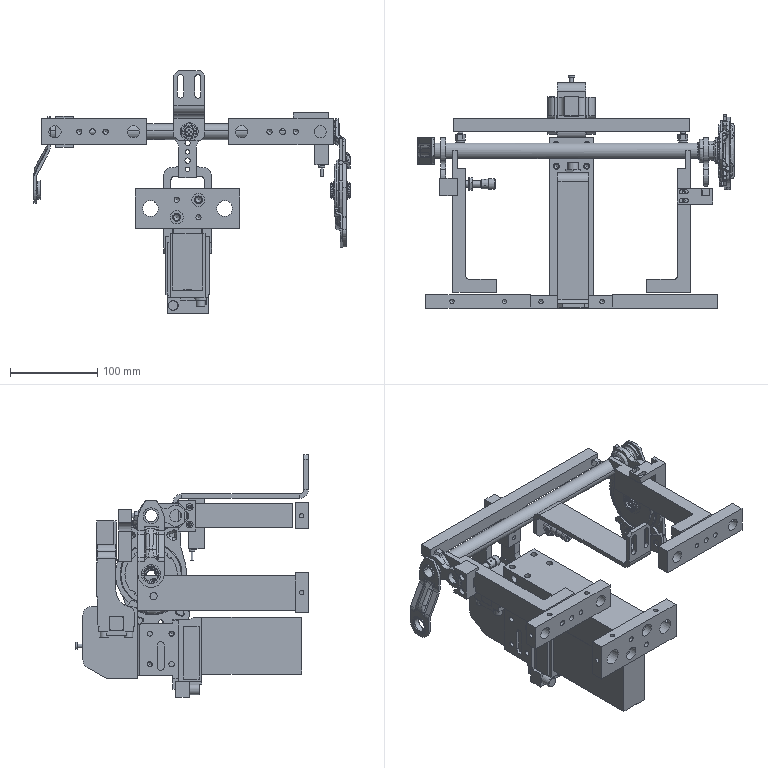Part | NX | features BREP 45 | 53 solids | 3306 faces | volume 1671214 mm3 | cylinder 1202 | plane 1147 | spline 436 | cone 268 | torus 219 | sphere 34 | commonest cylinder face diameters 0.3 x169 0.6 x144 1 x74 4 x40 2 x38 3 x37